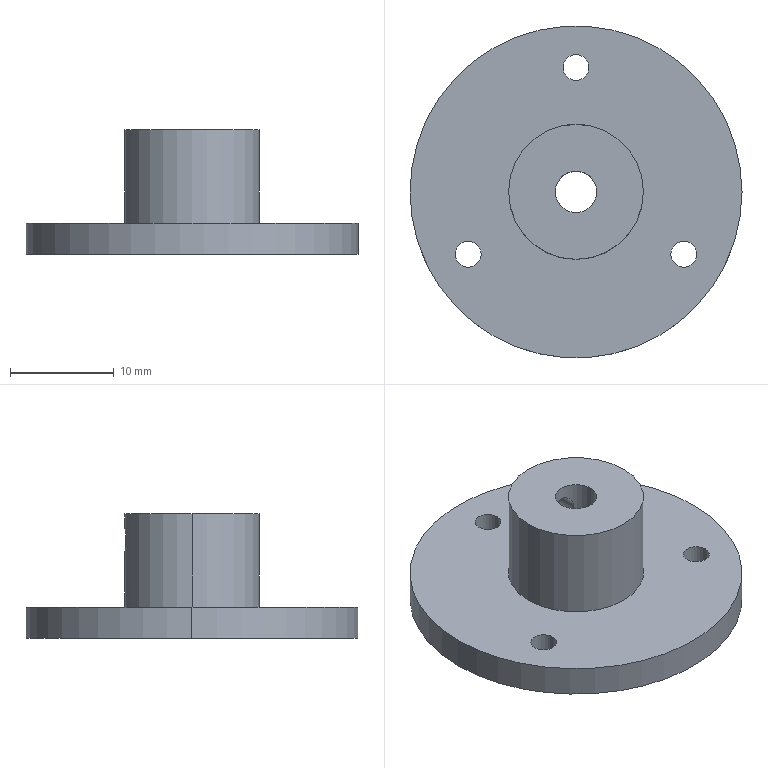Part | SolidWorks | features ICE 3, HoleWzd 2, Extrusion 1 | 1 solid | 17 faces | box 32 x 32 x 12 mm | volume 3390 mm3 | cylinder 14 | plane 3 | commonest cylinder face diameters 2.5 x8 4 x2 13 x2 32 x2
STEP:
#1=CARTESIAN_POINT('',(-1.25,12.,3.));
#2=VERTEX_POINT('',#1);
#3=CARTESIAN_POINT('',(1.25,12.,3.));
#4=VERTEX_POINT('',#3);
#5=CARTESIAN_POINT('',(0.,12.,3.));
#6=DIRECTION('',(0.,0.,1.));
#7=DIRECTION('',(1.,0.,0.));
#8=AXIS2_PLACEMENT_3D('',#5,#6,#7);
#9=CIRCLE('',#8,1.25);
#10=EDGE_CURVE('',#2,#4,#9,.T.);
#11=ORIENTED_EDGE('',*,*,#10,.T.);
#12=CARTESIAN_POINT('',(1.25,12.,0.));
#13=VERTEX_POINT('',#12);
#14=CARTESIAN_POINT('',(1.25,12.,0.));
#15=DIRECTION('',(0.,0.,-1.));
#16=VECTOR('',#15,1000.);
#17=LINE('',#14,#16);
#18=EDGE_CURVE('',#4,#13,#17,.T.);
#19=ORIENTED_EDGE('',*,*,#18,.T.);
#20=CARTESIAN_POINT('',(-1.25,12.,0.));
#21=VERTEX_POINT('',#20);
#22=CARTESIAN_POINT('',(0.,12.,0.));
#23=DIRECTION('',(0.,0.,-1.));
#24=DIRECTION('',(-1.,0.,0.));
#25=AXIS2_PLACEMENT_3D('',#22,#23,#24);
#26=CIRCLE('',#25,1.25);
#27=EDGE_CURVE('',#13,#21,#26,.T.);
#28=ORIENTED_EDGE('',*,*,#27,.T.);
#29=CARTESIAN_POINT('',(-1.25,12.,0.));
#30=DIRECTION('',(0.,0.,-1.));
#31=VECTOR('',#30,1000.);
#32=LINE('',#29,#31);
#33=EDGE_CURVE('',#2,#21,#32,.T.);
#34=ORIENTED_EDGE('',*,*,#33,.F.);
#35=EDGE_LOOP('',(#11,#19,#28,#34));
#36=FACE_OUTER_BOUND('',#35,.T.);
#37=CARTESIAN_POINT('',(0.,12.,0.));
#38=DIRECTION('',(0.,0.,-1.));
#39=DIRECTION('',(-1.,0.,0.));
#40=AXIS2_PLACEMENT_3D('',#37,#38,#39);
#41=CYLINDRICAL_SURFACE('',#40,1.25);
#42=ADVANCED_FACE('',(#36),#41,.F.);
#43=CARTESIAN_POINT('',(9.142,-6.,3.));
#44=VERTEX_POINT('',#43);
#45=CARTESIAN_POINT('',(11.642,-6.,3.));
#46=VERTEX_POINT('',#45);
#47=CARTESIAN_POINT('',(10.392,-6.,3.));
#48=DIRECTION('',(0.,0.,1.));
#49=DIRECTION('',(1.,0.,0.));
#50=AXIS2_PLACEMENT_3D('',#47,#48,#49);
#51=CIRCLE('',#50,1.25);
#52=EDGE_CURVE('',#44,#46,#51,.T.);
#53=ORIENTED_EDGE('',*,*,#52,.T.);
#54=CARTESIAN_POINT('',(11.642,-6.,0.));
#55=VERTEX_POINT('',#54);
#56=CARTESIAN_POINT('',(11.642,-6.,0.));
#57=DIRECTION('',(0.,0.,-1.));
#58=VECTOR('',#57,1000.);
#59=LINE('',#56,#58);
#60=EDGE_CURVE('',#46,#55,#59,.T.);
#61=ORIENTED_EDGE('',*,*,#60,.T.);
#62=CARTESIAN_POINT('',(9.142,-6.,0.));
#63=VERTEX_POINT('',#62);
#64=CARTESIAN_POINT('',(10.392,-6.,0.));
#65=DIRECTION('',(0.,0.,-1.));
#66=DIRECTION('',(-1.,0.,0.));
#67=AXIS2_PLACEMENT_3D('',#64,#65,#66);
#68=CIRCLE('',#67,1.25);
#69=EDGE_CURVE('',#55,#63,#68,.T.);
#70=ORIENTED_EDGE('',*,*,#69,.T.);
#71=CARTESIAN_POINT('',(9.142,-6.,0.));
#72=DIRECTION('',(0.,0.,-1.));
#73=VECTOR('',#72,1000.);
#74=LINE('',#71,#73);
#75=EDGE_CURVE('',#44,#63,#74,.T.);
#76=ORIENTED_EDGE('',*,*,#75,.F.);
#77=EDGE_LOOP('',(#53,#61,#70,#76));
#78=FACE_OUTER_BOUND('',#77,.T.);
#79=CARTESIAN_POINT('',(10.392,-6.,0.));
#80=DIRECTION('',(0.,0.,-1.));
#81=DIRECTION('',(-1.,0.,0.));
#82=AXIS2_PLACEMENT_3D('',#79,#80,#81);
#83=CYLINDRICAL_SURFACE('',#82,1.25);
#84=ADVANCED_FACE('',(#78),#83,.F.);
#85=CARTESIAN_POINT('',(-11.642,-6.,3.));
#86=VERTEX_POINT('',#85);
#87=CARTESIAN_POINT('',(-9.142,-6.,3.));
#88=VERTEX_POINT('',#87);
#89=CARTESIAN_POINT('',(-10.392,-6.,3.));
#90=DIRECTION('',(0.,0.,1.));
#91=DIRECTION('',(1.,0.,0.));
#92=AXIS2_PLACEMENT_3D('',#89,#90,#91);
#93=CIRCLE('',#92,1.25);
#94=EDGE_CURVE('',#86,#88,#93,.T.);
#95=ORIENTED_EDGE('',*,*,#94,.T.);
#96=CARTESIAN_POINT('',(-9.142,-6.,0.));
#97=VERTEX_POINT('',#96);
#98=CARTESIAN_POINT('',(-9.142,-6.,0.));
#99=DIRECTION('',(0.,0.,-1.));
#100=VECTOR('',#99,1000.);
#101=LINE('',#98,#100);
#102=EDGE_CURVE('',#88,#97,#101,.T.);
#103=ORIENTED_EDGE('',*,*,#102,.T.);
#104=CARTESIAN_POINT('',(-11.642,-6.,0.));
#105=VERTEX_POINT('',#104);
#106=CARTESIAN_POINT('',(-10.392,-6.,0.));
#107=DIRECTION('',(0.,0.,-1.));
#108=DIRECTION('',(-1.,0.,0.));
#109=AXIS2_PLACEMENT_3D('',#106,#107,#108);
#110=CIRCLE('',#109,1.25);
#111=EDGE_CURVE('',#97,#105,#110,.T.);
#112=ORIENTED_EDGE('',*,*,#111,.T.);
#113=CARTESIAN_POINT('',(-11.642,-6.,0.));
#114=DIRECTION('',(0.,0.,-1.));
#115=VECTOR('',#114,1000.);
#116=LINE('',#113,#115);
#117=EDGE_CURVE('',#86,#105,#116,.T.);
#118=ORIENTED_EDGE('',*,*,#117,.F.);
#119=EDGE_LOOP('',(#95,#103,#112,#118));
#120=FACE_OUTER_BOUND('',#119,.T.);
#121=CARTESIAN_POINT('',(-10.392,-6.,0.));
#122=DIRECTION('',(0.,0.,-1.));
#123=DIRECTION('',(-1.,0.,0.));
#124=AXIS2_PLACEMENT_3D('',#121,#122,#123);
#125=CYLINDRICAL_SURFACE('',#124,1.25);
#126=ADVANCED_FACE('',(#120),#125,.F.);
#127=CARTESIAN_POINT('',(0.,6.5,10.75));
#128=VERTEX_POINT('',#127);
#129=CARTESIAN_POINT('',(0.,6.5,8.25));
#130=VERTEX_POINT('',#129);
#131=CARTESIAN_POINT('',(0.,6.5,10.75));
#132=CARTESIAN_POINT('',(-0.1633,6.5,10.75));
#133=CARTESIAN_POINT('',(-0.3282,6.493,10.717));
#134=CARTESIAN_POINT('',(-0.6291,6.471,10.592));
#135=CARTESIAN_POINT('',(-0.7681,6.456,10.5));
#136=CARTESIAN_POINT('',(-0.9987,6.424,10.269));
#137=CARTESIAN_POINT('',(-1.091,6.408,10.131));
#138=CARTESIAN_POINT('',(-1.217,6.385,9.828));
#139=CARTESIAN_POINT('',(-1.25,6.379,9.666));
#140=CARTESIAN_POINT('',(-1.25,6.379,9.336));
#141=CARTESIAN_POINT('',(-1.217,6.385,9.173));
#142=CARTESIAN_POINT('',(-1.092,6.408,8.87));
#143=CARTESIAN_POINT('',(-0.9993,6.424,8.732));
#144=CARTESIAN_POINT('',(-0.7696,6.455,8.502));
#145=CARTESIAN_POINT('',(-0.6305,6.471,8.408));
#146=CARTESIAN_POINT('',(-0.3299,6.493,8.283));
#147=CARTESIAN_POINT('',(-0.1656,6.5,8.25));
#148=CARTESIAN_POINT('',(0.,6.5,8.25));
#149=B_SPLINE_CURVE_WITH_KNOTS('',3,(#131,#132,#133,#134,#135,#136,#137,#138,#139,#140,#141,#142,#143,#144,#145,#146,#147,#148),.UNSPECIFIED.,.F.,.F.,(4,2,2,2,2,2,2,2,4),(0.003917,0.004407,0.004896,0.005386,0.005875,0.006365,0.006854,0.007344,0.007833),.UNSPECIFIED.);
#150=EDGE_CURVE('',#128,#130,#149,.T.);
#151=ORIENTED_EDGE('',*,*,#150,.F.);
#152=CARTESIAN_POINT('',(0.,2.,10.75));
#153=VERTEX_POINT('',#152);
#154=CARTESIAN_POINT('',(0.,0.,10.75));
#155=DIRECTION('',(0.,-1.,0.));
#156=VECTOR('',#155,1000.);
#157=LINE('',#154,#156);
#158=EDGE_CURVE('',#128,#153,#157,.T.);
#159=ORIENTED_EDGE('',*,*,#158,.T.);
#160=CARTESIAN_POINT('',(0.,2.,8.25));
#161=VERTEX_POINT('',#160);
#162=CARTESIAN_POINT('',(0.,2.,8.25));
#163=CARTESIAN_POINT('',(-0.08511,2.,8.25));
#164=CARTESIAN_POINT('',(-0.1684,1.995,8.259));
#165=CARTESIAN_POINT('',(-0.3316,1.974,8.292));
#166=CARTESIAN_POINT('',(-0.4122,1.959,8.317));
#167=CARTESIAN_POINT('',(-0.6385,1.902,8.413));
#168=CARTESIAN_POINT('',(-0.7738,1.848,8.506));
#169=CARTESIAN_POINT('',(-0.9977,1.738,8.73));
#170=CARTESIAN_POINT('',(-1.088,1.68,8.864));
#171=CARTESIAN_POINT('',(-1.214,1.591,9.162));
#172=CARTESIAN_POINT('',(-1.25,1.561,9.33));
#173=CARTESIAN_POINT('',(-1.25,1.561,9.669));
#174=CARTESIAN_POINT('',(-1.215,1.591,9.836));
#175=CARTESIAN_POINT('',(-1.089,1.68,10.135));
#176=CARTESIAN_POINT('',(-0.9982,1.738,10.269));
#177=CARTESIAN_POINT('',(-0.7723,1.849,10.496));
#178=CARTESIAN_POINT('',(-0.6398,1.901,10.587));
#179=CARTESIAN_POINT('',(-0.4108,1.959,10.683));
#180=CARTESIAN_POINT('',(-0.332,1.974,10.708));
#181=CARTESIAN_POINT('',(-0.1695,1.994,10.741));
#182=CARTESIAN_POINT('',(-0.0845,2.,10.75));
#183=CARTESIAN_POINT('',(0.,2.,10.75));
#184=B_SPLINE_CURVE_WITH_KNOTS('',3,(#162,#163,#164,#165,#166,#167,#168,#169,#170,#171,#172,#173,#174,#175,#176,#177,#178,#179,#180,#181,#182,#183),.UNSPECIFIED.,.F.,.F.,(4,2,2,2,2,2,2,2,2,2,4),(0.,0.0002513,0.0005026,0.001005,0.001508,0.002011,0.002513,0.003016,0.003518,0.00377,0.004021),.UNSPECIFIED.);
#185=EDGE_CURVE('',#161,#153,#184,.T.);
#186=ORIENTED_EDGE('',*,*,#185,.F.);
#187=CARTESIAN_POINT('',(0.,0.,8.25));
#188=DIRECTION('',(0.,-1.,0.));
#189=VECTOR('',#188,1000.);
#190=LINE('',#187,#189);
#191=EDGE_CURVE('',#130,#161,#190,.T.);
#192=ORIENTED_EDGE('',*,*,#191,.F.);
#193=EDGE_LOOP('',(#151,#159,#186,#192));
#194=FACE_OUTER_BOUND('',#193,.T.);
#195=CARTESIAN_POINT('',(0.,0.,9.5));
#196=DIRECTION('',(0.,-1.,0.));
#197=DIRECTION('',(0.,0.,-1.));
#198=AXIS2_PLACEMENT_3D('',#195,#196,#197);
#199=CYLINDRICAL_SURFACE('',#198,1.25);
#200=ADVANCED_FACE('',(#194),#199,.F.);
#201=CARTESIAN_POINT('',(-2.,0.,12.));
#202=VERTEX_POINT('',#201);
#203=CARTESIAN_POINT('',(2.,0.,12.));
#204=VERTEX_POINT('',#203);
#205=CARTESIAN_POINT('',(0.,0.,12.));
#206=DIRECTION('',(0.,0.,1.));
#207=DIRECTION('',(1.,0.,0.));
#208=AXIS2_PLACEMENT_3D('',#205,#206,#207);
#209=CIRCLE('',#208,2.);
#210=EDGE_CURVE('',#202,#204,#209,.T.);
#211=ORIENTED_EDGE('',*,*,#210,.T.);
#212=CARTESIAN_POINT('',(2.,0.,0.));
#213=VERTEX_POINT('',#212);
#214=CARTESIAN_POINT('',(2.,0.,22.));
#215=DIRECTION('',(0.,0.,-1.));
#216=VECTOR('',#215,1000.);
#217=LINE('',#214,#216);
#218=EDGE_CURVE('',#204,#213,#217,.T.);
#219=ORIENTED_EDGE('',*,*,#218,.T.);
#220=CARTESIAN_POINT('',(-2.,0.,0.));
#221=VERTEX_POINT('',#220);
#222=CARTESIAN_POINT('',(0.,0.,0.));
#223=DIRECTION('',(0.,0.,-1.));
#224=DIRECTION('',(-1.,0.,0.));
#225=AXIS2_PLACEMENT_3D('',#222,#223,#224);
#226=CIRCLE('',#225,2.);
#227=EDGE_CURVE('',#213,#221,#226,.T.);
#228=ORIENTED_EDGE('',*,*,#227,.T.);
#229=CARTESIAN_POINT('',(-2.,0.,22.));
#230=DIRECTION('',(0.,0.,-1.));
#231=VECTOR('',#230,1000.);
#232=LINE('',#229,#231);
#233=EDGE_CURVE('',#202,#221,#232,.T.);
#234=ORIENTED_EDGE('',*,*,#233,.F.);
#235=EDGE_LOOP('',(#211,#219,#228,#234));
#236=FACE_OUTER_BOUND('',#235,.T.);
#237=CARTESIAN_POINT('',(0.,0.,22.));
#238=DIRECTION('',(0.,0.,-1.));
#239=DIRECTION('',(-1.,0.,0.));
#240=AXIS2_PLACEMENT_3D('',#237,#238,#239);
#241=CYLINDRICAL_SURFACE('',#240,2.);
#242=ADVANCED_FACE('',(#236),#241,.F.);
#243=CARTESIAN_POINT('',(0.,6.5,8.25));
#244=CARTESIAN_POINT('',(0.1656,6.5,8.25));
#245=CARTESIAN_POINT('',(0.3281,6.493,8.283));
#246=CARTESIAN_POINT('',(0.6307,6.471,8.408));
#247=CARTESIAN_POINT('',(0.7691,6.455,8.501));
#248=CARTESIAN_POINT('',(0.9991,6.424,8.731));
#249=CARTESIAN_POINT('',(1.092,6.408,8.871));
#250=CARTESIAN_POINT('',(1.217,6.385,9.171));
#251=CARTESIAN_POINT('',(1.25,6.379,9.336));
#252=CARTESIAN_POINT('',(1.25,6.379,9.581));
#253=CARTESIAN_POINT('',(1.242,6.38,9.664));
#254=CARTESIAN_POINT('',(1.21,6.386,9.825));
#255=CARTESIAN_POINT('',(1.186,6.391,9.903));
#256=CARTESIAN_POINT('',(1.092,6.408,10.13));
#257=CARTESIAN_POINT('',(1.,6.424,10.268));
#258=CARTESIAN_POINT('',(0.7676,6.456,10.5));
#259=CARTESIAN_POINT('',(0.6299,6.471,10.592));
#260=CARTESIAN_POINT('',(0.3277,6.494,10.717));
#261=CARTESIAN_POINT('',(0.1634,6.5,10.75));
#262=CARTESIAN_POINT('',(0.,6.5,10.75));
#263=B_SPLINE_CURVE_WITH_KNOTS('',3,(#243,#244,#245,#246,#247,#248,#249,#250,#251,#252,#253,#254,#255,#256,#257,#258,#259,#260,#261,#262),.UNSPECIFIED.,.F.,.F.,(4,2,2,2,2,2,2,2,2,4),(0.,0.0004897,0.0009793,0.001469,0.001959,0.002203,0.002448,0.002938,0.003428,0.003917),.UNSPECIFIED.);
#264=EDGE_CURVE('',#130,#128,#263,.T.);
#265=ORIENTED_EDGE('',*,*,#264,.T.);
#266=ORIENTED_EDGE('',*,*,#150,.T.);
#267=EDGE_LOOP('',(#265,#266));
#268=FACE_BOUND('',#267,.T.);
#269=CARTESIAN_POINT('',(6.5,0.,12.));
#270=VERTEX_POINT('',#269);
#271=CARTESIAN_POINT('',(-6.5,0.,12.));
#272=VERTEX_POINT('',#271);
#273=CARTESIAN_POINT('',(0.,0.,12.));
#274=DIRECTION('',(0.,0.,1.));
#275=DIRECTION('',(1.,0.,0.));
#276=AXIS2_PLACEMENT_3D('',#273,#274,#275);
#277=CIRCLE('',#276,6.5);
#278=EDGE_CURVE('',#270,#272,#277,.T.);
#279=ORIENTED_EDGE('',*,*,#278,.F.);
#280=CARTESIAN_POINT('',(6.5,0.,3.));
#281=VERTEX_POINT('',#280);
#282=CARTESIAN_POINT('',(6.5,0.,12.));
#283=DIRECTION('',(0.,0.,-1.));
#284=VECTOR('',#283,1000.);
#285=LINE('',#282,#284);
#286=EDGE_CURVE('',#270,#281,#285,.T.);
#287=ORIENTED_EDGE('',*,*,#286,.T.);
#288=CARTESIAN_POINT('',(-6.5,0.,3.));
#289=VERTEX_POINT('',#288);
#290=CARTESIAN_POINT('',(0.,0.,3.));
#291=DIRECTION('',(0.,0.,1.));
#292=DIRECTION('',(1.,0.,0.));
#293=AXIS2_PLACEMENT_3D('',#290,#291,#292);
#294=CIRCLE('',#293,6.5);
#295=EDGE_CURVE('',#281,#289,#294,.T.);
#296=ORIENTED_EDGE('',*,*,#295,.T.);
#297=CARTESIAN_POINT('',(-6.5,0.,12.));
#298=DIRECTION('',(0.,0.,-1.));
#299=VECTOR('',#298,1000.);
#300=LINE('',#297,#299);
#301=EDGE_CURVE('',#272,#289,#300,.T.);
#302=ORIENTED_EDGE('',*,*,#301,.F.);
#303=EDGE_LOOP('',(#279,#287,#296,#302));
#304=FACE_OUTER_BOUND('',#303,.T.);
#305=CARTESIAN_POINT('',(0.,0.,12.));
#306=DIRECTION('',(0.,0.,-1.));
#307=DIRECTION('',(-1.,0.,0.));
#308=AXIS2_PLACEMENT_3D('',#305,#306,#307);
#309=CYLINDRICAL_SURFACE('',#308,6.5);
#310=ADVANCED_FACE('',(#268,#304),#309,.T.);
#311=CARTESIAN_POINT('',(16.,0.,3.));
#312=VERTEX_POINT('',#311);
#313=CARTESIAN_POINT('',(-16.,0.,3.));
#314=VERTEX_POINT('',#313);
#315=CARTESIAN_POINT('',(0.,0.,3.));
#316=DIRECTION('',(0.,0.,1.));
#317=DIRECTION('',(1.,0.,0.));
#318=AXIS2_PLACEMENT_3D('',#315,#316,#317);
#319=CIRCLE('',#318,16.);
#320=EDGE_CURVE('',#312,#314,#319,.T.);
#321=ORIENTED_EDGE('',*,*,#320,.F.);
#322=CARTESIAN_POINT('',(16.,0.,0.));
#323=VERTEX_POINT('',#322);
#324=CARTESIAN_POINT('',(16.,0.,3.));
#325=DIRECTION('',(0.,0.,-1.));
#326=VECTOR('',#325,1000.);
#327=LINE('',#324,#326);
#328=EDGE_CURVE('',#312,#323,#327,.T.);
#329=ORIENTED_EDGE('',*,*,#328,.T.);
#330=CARTESIAN_POINT('',(-16.,0.,0.));
#331=VERTEX_POINT('',#330);
#332=CARTESIAN_POINT('',(0.,0.,0.));
#333=DIRECTION('',(0.,0.,1.));
#334=DIRECTION('',(1.,0.,0.));
#335=AXIS2_PLACEMENT_3D('',#332,#333,#334);
#336=CIRCLE('',#335,16.);
#337=EDGE_CURVE('',#323,#331,#336,.T.);
#338=ORIENTED_EDGE('',*,*,#337,.T.);
#339=CARTESIAN_POINT('',(-16.,0.,3.));
#340=DIRECTION('',(0.,0.,-1.));
#341=VECTOR('',#340,1000.);
#342=LINE('',#339,#341);
#343=EDGE_CURVE('',#314,#331,#342,.T.);
#344=ORIENTED_EDGE('',*,*,#343,.F.);
#345=EDGE_LOOP('',(#321,#329,#338,#344));
#346=FACE_OUTER_BOUND('',#345,.T.);
#347=CARTESIAN_POINT('',(0.,0.,3.));
#348=DIRECTION('',(0.,0.,-1.));
#349=DIRECTION('',(-1.,0.,0.));
#350=AXIS2_PLACEMENT_3D('',#347,#348,#349);
#351=CYLINDRICAL_SURFACE('',#350,16.);
#352=ADVANCED_FACE('',(#346),#351,.T.);
#353=CARTESIAN_POINT('',(0.,12.,0.));
#354=DIRECTION('',(0.,0.,-1.));
#355=DIRECTION('',(-1.,0.,0.));
#356=AXIS2_PLACEMENT_3D('',#353,#354,#355);
#357=CIRCLE('',#356,1.25);
#358=EDGE_CURVE('',#21,#13,#357,.T.);
#359=ORIENTED_EDGE('',*,*,#358,.F.);
#360=ORIENTED_EDGE('',*,*,#27,.F.);
#361=EDGE_LOOP('',(#359,#360));
#362=FACE_BOUND('',#361,.T.);
#363=CARTESIAN_POINT('',(10.392,-6.,0.));
#364=DIRECTION('',(0.,0.,-1.));
#365=DIRECTION('',(-1.,0.,0.));
#366=AXIS2_PLACEMENT_3D('',#363,#364,#365);
#367=CIRCLE('',#366,1.25);
#368=EDGE_CURVE('',#63,#55,#367,.T.);
#369=ORIENTED_EDGE('',*,*,#368,.F.);
#370=ORIENTED_EDGE('',*,*,#69,.F.);
#371=EDGE_LOOP('',(#369,#370));
#372=FACE_BOUND('',#371,.T.);
#373=CARTESIAN_POINT('',(0.,0.,0.));
#374=DIRECTION('',(0.,0.,1.));
#375=DIRECTION('',(1.,0.,0.));
#376=AXIS2_PLACEMENT_3D('',#373,#374,#375);
#377=CIRCLE('',#376,16.);
#378=EDGE_CURVE('',#331,#323,#377,.T.);
#379=ORIENTED_EDGE('',*,*,#378,.F.);
#380=ORIENTED_EDGE('',*,*,#337,.F.);
#381=EDGE_LOOP('',(#379,#380));
#382=FACE_OUTER_BOUND('',#381,.T.);
#383=CARTESIAN_POINT('',(0.,0.,0.));
#384=DIRECTION('',(0.,0.,-1.));
#385=DIRECTION('',(-1.,0.,0.));
#386=AXIS2_PLACEMENT_3D('',#383,#384,#385);
#387=CIRCLE('',#386,2.);
#388=EDGE_CURVE('',#221,#213,#387,.T.);
#389=ORIENTED_EDGE('',*,*,#388,.F.);
#390=ORIENTED_EDGE('',*,*,#227,.F.);
#391=EDGE_LOOP('',(#389,#390));
#392=FACE_BOUND('',#391,.T.);
#393=CARTESIAN_POINT('',(-10.392,-6.,0.));
#394=DIRECTION('',(0.,0.,-1.));
#395=DIRECTION('',(-1.,0.,0.));
#396=AXIS2_PLACEMENT_3D('',#393,#394,#395);
#397=CIRCLE('',#396,1.25);
#398=EDGE_CURVE('',#105,#97,#397,.T.);
#399=ORIENTED_EDGE('',*,*,#398,.F.);
#400=ORIENTED_EDGE('',*,*,#111,.F.);
#401=EDGE_LOOP('',(#399,#400));
#402=FACE_BOUND('',#401,.T.);
#403=CARTESIAN_POINT('',(0.,0.,0.));
#404=DIRECTION('',(0.,0.,1.));
#405=DIRECTION('',(1.,0.,0.));
#406=AXIS2_PLACEMENT_3D('',#403,#404,#405);
#407=PLANE('',#406);
#408=ADVANCED_FACE('',(#362,#372,#382,#392,#402),#407,.F.);
#409=ORIENTED_EDGE('',*,*,#328,.F.);
#410=CARTESIAN_POINT('',(0.,0.,3.));
#411=DIRECTION('',(0.,0.,1.));
#412=DIRECTION('',(1.,0.,0.));
#413=AXIS2_PLACEMENT_3D('',#410,#411,#412);
#414=CIRCLE('',#413,16.);
#415=EDGE_CURVE('',#314,#312,#414,.T.);
#416=ORIENTED_EDGE('',*,*,#415,.F.);
#417=ORIENTED_EDGE('',*,*,#343,.T.);
#418=ORIENTED_EDGE('',*,*,#378,.T.);
#419=EDGE_LOOP('',(#409,#416,#417,#418));
#420=FACE_OUTER_BOUND('',#419,.T.);
#421=CARTESIAN_POINT('',(0.,0.,3.));
#422=DIRECTION('',(0.,0.,-1.));
#423=DIRECTION('',(-1.,0.,0.));
#424=AXIS2_PLACEMENT_3D('',#421,#422,#423);
#425=CYLINDRICAL_SURFACE('',#424,16.);
#426=ADVANCED_FACE('',(#420),#425,.T.);
#427=ORIENTED_EDGE('',*,*,#10,.F.);
#428=CARTESIAN_POINT('',(0.,12.,3.));
#429=DIRECTION('',(0.,0.,1.));
#430=DIRECTION('',(1.,0.,0.));
#431=AXIS2_PLACEMENT_3D('',#428,#429,#430);
#432=CIRCLE('',#431,1.25);
#433=EDGE_CURVE('',#4,#2,#432,.T.);
#434=ORIENTED_EDGE('',*,*,#433,.F.);
#435=EDGE_LOOP('',(#427,#434));
#436=FACE_BOUND('',#435,.T.);
#437=ORIENTED_EDGE('',*,*,#52,.F.);
#438=CARTESIAN_POINT('',(10.392,-6.,3.));
#439=DIRECTION('',(0.,0.,1.));
#440=DIRECTION('',(1.,0.,0.));
#441=AXIS2_PLACEMENT_3D('',#438,#439,#440);
#442=CIRCLE('',#441,1.25);
#443=EDGE_CURVE('',#46,#44,#442,.T.);
#444=ORIENTED_EDGE('',*,*,#443,.F.);
#445=EDGE_LOOP('',(#437,#444));
#446=FACE_BOUND('',#445,.T.);
#447=ORIENTED_EDGE('',*,*,#94,.F.);
#448=CARTESIAN_POINT('',(-10.392,-6.,3.));
#449=DIRECTION('',(0.,0.,1.));
#450=DIRECTION('',(1.,0.,0.));
#451=AXIS2_PLACEMENT_3D('',#448,#449,#450);
#452=CIRCLE('',#451,1.25);
#453=EDGE_CURVE('',#88,#86,#452,.T.);
#454=ORIENTED_EDGE('',*,*,#453,.F.);
#455=EDGE_LOOP('',(#447,#454));
#456=FACE_BOUND('',#455,.T.);
#457=CARTESIAN_POINT('',(0.,0.,3.));
#458=DIRECTION('',(0.,0.,1.));
#459=DIRECTION('',(1.,0.,0.));
#460=AXIS2_PLACEMENT_3D('',#457,#458,#459);
#461=CIRCLE('',#460,6.5);
#462=EDGE_CURVE('',#289,#281,#461,.T.);
#463=ORIENTED_EDGE('',*,*,#462,.F.);
#464=ORIENTED_EDGE('',*,*,#295,.F.);
#465=EDGE_LOOP('',(#463,#464));
#466=FACE_BOUND('',#465,.T.);
#467=ORIENTED_EDGE('',*,*,#415,.T.);
#468=ORIENTED_EDGE('',*,*,#320,.T.);
#469=EDGE_LOOP('',(#467,#468));
#470=FACE_OUTER_BOUND('',#469,.T.);
#471=CARTESIAN_POINT('',(0.,0.,3.));
#472=DIRECTION('',(0.,0.,1.));
#473=DIRECTION('',(1.,0.,0.));
#474=AXIS2_PLACEMENT_3D('',#471,#472,#473);
#475=PLANE('',#474);
#476=ADVANCED_FACE('',(#436,#446,#456,#466,#470),#475,.T.);
#477=ORIENTED_EDGE('',*,*,#286,.F.);
#478=CARTESIAN_POINT('',(0.,0.,12.));
#479=DIRECTION('',(0.,0.,1.));
#480=DIRECTION('',(1.,0.,0.));
#481=AXIS2_PLACEMENT_3D('',#478,#479,#480);
#482=CIRCLE('',#481,6.5);
#483=EDGE_CURVE('',#272,#270,#482,.T.);
#484=ORIENTED_EDGE('',*,*,#483,.F.);
#485=ORIENTED_EDGE('',*,*,#301,.T.);
#486=ORIENTED_EDGE('',*,*,#462,.T.);
#487=EDGE_LOOP('',(#477,#484,#485,#486));
#488=FACE_OUTER_BOUND('',#487,.T.);
#489=CARTESIAN_POINT('',(0.,0.,12.));
#490=DIRECTION('',(0.,0.,-1.));
#491=DIRECTION('',(-1.,0.,0.));
#492=AXIS2_PLACEMENT_3D('',#489,#490,#491);
#493=CYLINDRICAL_SURFACE('',#492,6.5);
#494=ADVANCED_FACE('',(#488),#493,.T.);
#495=ORIENTED_EDGE('',*,*,#210,.F.);
#496=CARTESIAN_POINT('',(0.,0.,12.));
#497=DIRECTION('',(0.,0.,1.));
#498=DIRECTION('',(1.,0.,0.));
#499=AXIS2_PLACEMENT_3D('',#496,#497,#498);
#500=CIRCLE('',#499,2.);
#501=EDGE_CURVE('',#204,#202,#500,.T.);
#502=ORIENTED_EDGE('',*,*,#501,.F.);
#503=EDGE_LOOP('',(#495,#502));
#504=FACE_BOUND('',#503,.T.);
#505=ORIENTED_EDGE('',*,*,#483,.T.);
#506=ORIENTED_EDGE('',*,*,#278,.T.);
#507=EDGE_LOOP('',(#505,#506));
#508=FACE_OUTER_BOUND('',#507,.T.);
#509=CARTESIAN_POINT('',(0.,0.,12.));
#510=DIRECTION('',(0.,0.,1.));
#511=DIRECTION('',(1.,0.,0.));
#512=AXIS2_PLACEMENT_3D('',#509,#510,#511);
#513=PLANE('',#512);
#514=ADVANCED_FACE('',(#504,#508),#513,.T.);
#515=ORIENTED_EDGE('',*,*,#218,.F.);
#516=ORIENTED_EDGE('',*,*,#501,.T.);
#517=ORIENTED_EDGE('',*,*,#233,.T.);
#518=ORIENTED_EDGE('',*,*,#388,.T.);
#519=EDGE_LOOP('',(#515,#516,#517,#518));
#520=FACE_OUTER_BOUND('',#519,.T.);
#521=ORIENTED_EDGE('',*,*,#185,.T.);
#522=CARTESIAN_POINT('',(0.,2.,10.75));
#523=CARTESIAN_POINT('',(0.1686,2.,10.75));
#524=CARTESIAN_POINT('',(0.3364,1.978,10.715));
#525=CARTESIAN_POINT('',(0.6379,1.902,10.587));
#526=CARTESIAN_POINT('',(0.773,1.849,10.495));
#527=CARTESIAN_POINT('',(0.9982,1.738,10.269));
#528=CARTESIAN_POINT('',(1.088,1.68,10.137));
#529=CARTESIAN_POINT('',(1.183,1.613,9.911));
#530=CARTESIAN_POINT('',(1.208,1.594,9.833));
#531=CARTESIAN_POINT('',(1.241,1.568,9.67));
#532=CARTESIAN_POINT('',(1.25,1.561,9.584));
#533=CARTESIAN_POINT('',(1.25,1.561,9.333));
#534=CARTESIAN_POINT('',(1.215,1.59,9.165));
#535=CARTESIAN_POINT('',(1.089,1.679,8.865));
#536=CARTESIAN_POINT('',(0.9979,1.738,8.731));
#537=CARTESIAN_POINT('',(0.8293,1.821,8.561));
#538=CARTESIAN_POINT('',(0.7682,1.848,8.511));
#539=CARTESIAN_POINT('',(0.6354,1.898,8.421));
#540=CARTESIAN_POINT('',(0.5628,1.921,8.381));
#541=CARTESIAN_POINT('',(0.4124,1.959,8.317));
#542=CARTESIAN_POINT('',(0.3341,1.974,8.293));
#543=CARTESIAN_POINT('',(0.1706,1.994,8.259));
#544=CARTESIAN_POINT('',(0.08492,2.,8.25));
#545=CARTESIAN_POINT('',(0.,2.,8.25));
#546=B_SPLINE_CURVE_WITH_KNOTS('',3,(#522,#523,#524,#525,#526,#527,#528,#529,#530,#531,#532,#533,#534,#535,#536,#537,#538,#539,#540,#541,#542,#543,#544,#545),.UNSPECIFIED.,.F.,.F.,(4,2,2,2,2,2,2,2,2,2,2,4),(0.004021,0.004522,0.005024,0.005525,0.005776,0.006027,0.006528,0.00703,0.007281,0.007531,0.007782,0.008033),.UNSPECIFIED.);
#547=EDGE_CURVE('',#153,#161,#546,.T.);
#548=ORIENTED_EDGE('',*,*,#547,.T.);
#549=EDGE_LOOP('',(#521,#548));
#550=FACE_BOUND('',#549,.T.);
#551=CARTESIAN_POINT('',(0.,0.,22.));
#552=DIRECTION('',(0.,0.,-1.));
#553=DIRECTION('',(-1.,0.,0.));
#554=AXIS2_PLACEMENT_3D('',#551,#552,#553);
#555=CYLINDRICAL_SURFACE('',#554,2.);
#556=ADVANCED_FACE('',(#520,#550),#555,.F.);
#557=ORIENTED_EDGE('',*,*,#158,.F.);
#558=ORIENTED_EDGE('',*,*,#264,.F.);
#559=ORIENTED_EDGE('',*,*,#191,.T.);
#560=ORIENTED_EDGE('',*,*,#547,.F.);
#561=EDGE_LOOP('',(#557,#558,#559,#560));
#562=FACE_OUTER_BOUND('',#561,.T.);
#563=CARTESIAN_POINT('',(0.,0.,9.5));
#564=DIRECTION('',(0.,-1.,0.));
#565=DIRECTION('',(0.,0.,-1.));
#566=AXIS2_PLACEMENT_3D('',#563,#564,#565);
#567=CYLINDRICAL_SURFACE('',#566,1.25);
#568=ADVANCED_FACE('',(#562),#567,.F.);
#569=ORIENTED_EDGE('',*,*,#102,.F.);
#570=ORIENTED_EDGE('',*,*,#453,.T.);
#571=ORIENTED_EDGE('',*,*,#117,.T.);
#572=ORIENTED_EDGE('',*,*,#398,.T.);
#573=EDGE_LOOP('',(#569,#570,#571,#572));
#574=FACE_OUTER_BOUND('',#573,.T.);
#575=CARTESIAN_POINT('',(-10.392,-6.,0.));
#576=DIRECTION('',(0.,0.,-1.));
#577=DIRECTION('',(-1.,0.,0.));
#578=AXIS2_PLACEMENT_3D('',#575,#576,#577);
#579=CYLINDRICAL_SURFACE('',#578,1.25);
#580=ADVANCED_FACE('',(#574),#579,.F.);
#581=ORIENTED_EDGE('',*,*,#60,.F.);
#582=ORIENTED_EDGE('',*,*,#443,.T.);
#583=ORIENTED_EDGE('',*,*,#75,.T.);
#584=ORIENTED_EDGE('',*,*,#368,.T.);
#585=EDGE_LOOP('',(#581,#582,#583,#584));
#586=FACE_OUTER_BOUND('',#585,.T.);
#587=CARTESIAN_POINT('',(10.392,-6.,0.));
#588=DIRECTION('',(0.,0.,-1.));
#589=DIRECTION('',(-1.,0.,0.));
#590=AXIS2_PLACEMENT_3D('',#587,#588,#589);
#591=CYLINDRICAL_SURFACE('',#590,1.25);
#592=ADVANCED_FACE('',(#586),#591,.F.);
#593=ORIENTED_EDGE('',*,*,#18,.F.);
#594=ORIENTED_EDGE('',*,*,#433,.T.);
#595=ORIENTED_EDGE('',*,*,#33,.T.);
#596=ORIENTED_EDGE('',*,*,#358,.T.);
#597=EDGE_LOOP('',(#593,#594,#595,#596));
#598=FACE_OUTER_BOUND('',#597,.T.);
#599=CARTESIAN_POINT('',(0.,12.,0.));
#600=DIRECTION('',(0.,0.,-1.));
#601=DIRECTION('',(-1.,0.,0.));
#602=AXIS2_PLACEMENT_3D('',#599,#600,#601);
#603=CYLINDRICAL_SURFACE('',#602,1.25);
#604=ADVANCED_FACE('',(#598),#603,.F.);
#605=CLOSED_SHELL('',(#42,#84,#126,#200,#242,#310,#352,#408,#426,#476,#494,#514,#556,#568,#580,#592,#604));
#606=MANIFOLD_SOLID_BREP('',#605);
#607=CARTESIAN_POINT('',(0.,0.,0.));
#608=DIRECTION('',(0.,0.,1.));
#609=DIRECTION('',(1.,0.,0.));
#610=AXIS2_PLACEMENT_3D('',#607,#608,#609);
#611=(LENGTH_UNIT()NAMED_UNIT(*)SI_UNIT(.MILLI.,.METRE.));
#612=UNCERTAINTY_MEASURE_WITH_UNIT(LENGTH_MEASURE(0.00001),#611,'','');
#613=(NAMED_UNIT(*)PLANE_ANGLE_UNIT()SI_UNIT($,.RADIAN.));
#614=(NAMED_UNIT(*)SI_UNIT($,.STERADIAN.)SOLID_ANGLE_UNIT());
#615=(GEOMETRIC_REPRESENTATION_CONTEXT(3)GLOBAL_UNCERTAINTY_ASSIGNED_CONTEXT((#612))GLOBAL_UNIT_ASSIGNED_CONTEXT((#611,#613,#614))REPRESENTATION_CONTEXT('',''));
#616=ADVANCED_BREP_SHAPE_REPRESENTATION('',(#606,#610),#615);